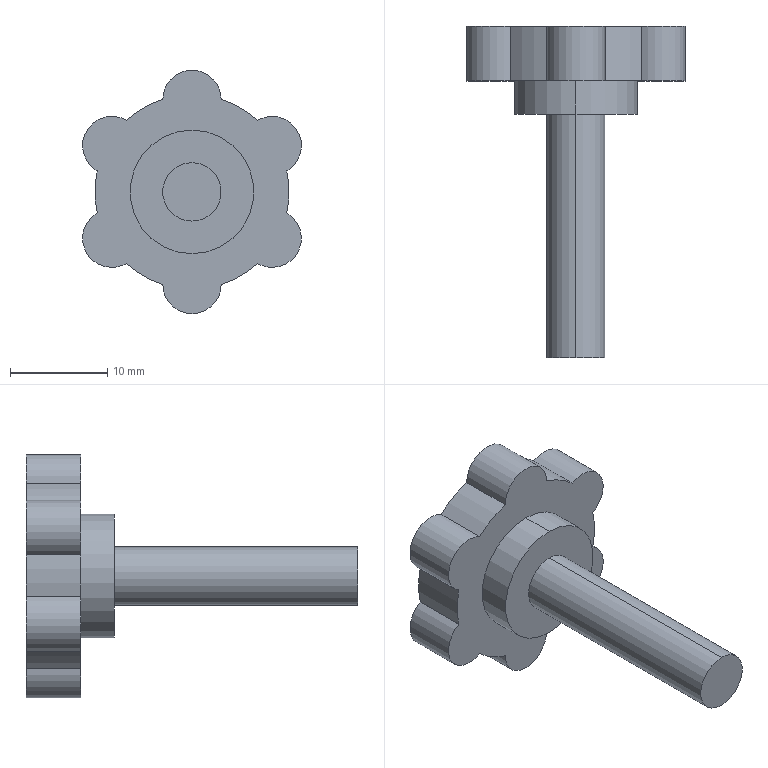Part | SolidWorks | features ICE 2, Extrusion 1 | 1 solid | 34 faces | box 22.455 x 34 x 25 mm | volume 3296 mm3 | cylinder 19 | plane 15 | commonest cylinder face diameters 6 x11 19.922 x6 12.7 x2
STEP:
#1=CARTESIAN_POINT('',(0.,-28.4,-3.));
#2=VERTEX_POINT('',#1);
#3=CARTESIAN_POINT('',(0.,-28.4,3.));
#4=VERTEX_POINT('',#3);
#5=CARTESIAN_POINT('',(0.,-28.4,0.));
#6=DIRECTION('',(0.,-1.,0.));
#7=DIRECTION('',(0.,0.,-1.));
#8=AXIS2_PLACEMENT_3D('',#5,#6,#7);
#9=CIRCLE('',#8,3.);
#10=EDGE_CURVE('',#2,#4,#9,.T.);
#11=ORIENTED_EDGE('',*,*,#10,.F.);
#12=CARTESIAN_POINT('',(0.,-3.4,-3.));
#13=VERTEX_POINT('',#12);
#14=CARTESIAN_POINT('',(0.,-28.4,-3.));
#15=DIRECTION('',(0.,1.,0.));
#16=VECTOR('',#15,1000.);
#17=LINE('',#14,#16);
#18=EDGE_CURVE('',#2,#13,#17,.T.);
#19=ORIENTED_EDGE('',*,*,#18,.T.);
#20=CARTESIAN_POINT('',(0.,-3.4,3.));
#21=VERTEX_POINT('',#20);
#22=CARTESIAN_POINT('',(0.,-3.4,0.));
#23=DIRECTION('',(0.,-1.,0.));
#24=DIRECTION('',(0.,0.,-1.));
#25=AXIS2_PLACEMENT_3D('',#22,#23,#24);
#26=CIRCLE('',#25,3.);
#27=EDGE_CURVE('',#13,#21,#26,.T.);
#28=ORIENTED_EDGE('',*,*,#27,.T.);
#29=CARTESIAN_POINT('',(0.,-28.4,3.));
#30=DIRECTION('',(0.,1.,0.));
#31=VECTOR('',#30,1000.);
#32=LINE('',#29,#31);
#33=EDGE_CURVE('',#4,#21,#32,.T.);
#34=ORIENTED_EDGE('',*,*,#33,.F.);
#35=EDGE_LOOP('',(#11,#19,#28,#34));
#36=FACE_OUTER_BOUND('',#35,.T.);
#37=CARTESIAN_POINT('',(0.,-28.4,0.));
#38=DIRECTION('',(0.,1.,0.));
#39=DIRECTION('',(0.,0.,1.));
#40=AXIS2_PLACEMENT_3D('',#37,#38,#39);
#41=CYLINDRICAL_SURFACE('',#40,3.);
#42=ADVANCED_FACE('',(#36),#41,.T.);
#43=CARTESIAN_POINT('',(0.,-3.4,-6.35));
#44=VERTEX_POINT('',#43);
#45=CARTESIAN_POINT('',(0.,-3.4,6.35));
#46=VERTEX_POINT('',#45);
#47=CARTESIAN_POINT('',(0.,-3.4,0.));
#48=DIRECTION('',(0.,-1.,0.));
#49=DIRECTION('',(0.,0.,-1.));
#50=AXIS2_PLACEMENT_3D('',#47,#48,#49);
#51=CIRCLE('',#50,6.35);
#52=EDGE_CURVE('',#44,#46,#51,.T.);
#53=ORIENTED_EDGE('',*,*,#52,.F.);
#54=CARTESIAN_POINT('',(0.,0.,-6.35));
#55=VERTEX_POINT('',#54);
#56=CARTESIAN_POINT('',(0.,-3.4,-6.35));
#57=DIRECTION('',(0.,1.,0.));
#58=VECTOR('',#57,1000.);
#59=LINE('',#56,#58);
#60=EDGE_CURVE('',#44,#55,#59,.T.);
#61=ORIENTED_EDGE('',*,*,#60,.T.);
#62=CARTESIAN_POINT('',(0.,0.,6.35));
#63=VERTEX_POINT('',#62);
#64=CARTESIAN_POINT('',(0.,0.,0.));
#65=DIRECTION('',(0.,-1.,0.));
#66=DIRECTION('',(0.,0.,1.));
#67=AXIS2_PLACEMENT_3D('',#64,#65,#66);
#68=CIRCLE('',#67,6.35);
#69=EDGE_CURVE('',#55,#63,#68,.T.);
#70=ORIENTED_EDGE('',*,*,#69,.T.);
#71=CARTESIAN_POINT('',(0.,-3.4,6.35));
#72=DIRECTION('',(0.,1.,0.));
#73=VECTOR('',#72,1000.);
#74=LINE('',#71,#73);
#75=EDGE_CURVE('',#46,#63,#74,.T.);
#76=ORIENTED_EDGE('',*,*,#75,.F.);
#77=EDGE_LOOP('',(#53,#61,#70,#76));
#78=FACE_OUTER_BOUND('',#77,.T.);
#79=CARTESIAN_POINT('',(0.,-3.4,0.));
#80=DIRECTION('',(0.,1.,0.));
#81=DIRECTION('',(0.,0.,1.));
#82=AXIS2_PLACEMENT_3D('',#79,#80,#81);
#83=CYLINDRICAL_SURFACE('',#82,6.35);
#84=ADVANCED_FACE('',(#78),#83,.T.);
#85=CARTESIAN_POINT('',(8.228,5.6,-7.751));
#86=VERTEX_POINT('',#85);
#87=CARTESIAN_POINT('',(6.728,5.6,-7.349));
#88=VERTEX_POINT('',#87);
#89=CARTESIAN_POINT('',(8.228,5.6,-4.751));
#90=DIRECTION('',(0.,1.,0.));
#91=DIRECTION('',(0.,0.,1.));
#92=AXIS2_PLACEMENT_3D('',#89,#90,#91);
#93=CIRCLE('',#92,3.);
#94=EDGE_CURVE('',#86,#88,#93,.T.);
#95=ORIENTED_EDGE('',*,*,#94,.F.);
#96=CARTESIAN_POINT('',(8.228,0.,-7.751));
#97=VERTEX_POINT('',#96);
#98=CARTESIAN_POINT('',(8.228,5.6,-7.751));
#99=DIRECTION('',(0.,-1.,0.));
#100=VECTOR('',#99,1000.);
#101=LINE('',#98,#100);
#102=EDGE_CURVE('',#86,#97,#101,.T.);
#103=ORIENTED_EDGE('',*,*,#102,.T.);
#104=CARTESIAN_POINT('',(6.728,0.,-7.349));
#105=VERTEX_POINT('',#104);
#106=CARTESIAN_POINT('',(8.228,0.,-4.751));
#107=DIRECTION('',(0.,1.,0.));
#108=DIRECTION('',(0.,0.,1.));
#109=AXIS2_PLACEMENT_3D('',#106,#107,#108);
#110=CIRCLE('',#109,3.);
#111=EDGE_CURVE('',#97,#105,#110,.T.);
#112=ORIENTED_EDGE('',*,*,#111,.T.);
#113=CARTESIAN_POINT('',(6.728,5.6,-7.349));
#114=DIRECTION('',(0.,-1.,0.));
#115=VECTOR('',#114,1000.);
#116=LINE('',#113,#115);
#117=EDGE_CURVE('',#88,#105,#116,.T.);
#118=ORIENTED_EDGE('',*,*,#117,.F.);
#119=EDGE_LOOP('',(#95,#103,#112,#118));
#120=FACE_OUTER_BOUND('',#119,.T.);
#121=CARTESIAN_POINT('',(8.228,5.6,-4.751));
#122=DIRECTION('',(0.,-1.,0.));
#123=DIRECTION('',(0.,0.,-1.));
#124=AXIS2_PLACEMENT_3D('',#121,#122,#123);
#125=CYLINDRICAL_SURFACE('',#124,3.);
#126=ADVANCED_FACE('',(#120),#125,.T.);
#127=CARTESIAN_POINT('',(-8.227,5.6,-7.749));
#128=VERTEX_POINT('',#127);
#129=CARTESIAN_POINT('',(-9.727,5.6,-2.151));
#130=VERTEX_POINT('',#129);
#131=CARTESIAN_POINT('',(-8.227,5.6,-4.749));
#132=DIRECTION('',(0.,1.,0.));
#133=DIRECTION('',(0.,0.,1.));
#134=AXIS2_PLACEMENT_3D('',#131,#132,#133);
#135=CIRCLE('',#134,3.);
#136=EDGE_CURVE('',#128,#130,#135,.T.);
#137=ORIENTED_EDGE('',*,*,#136,.F.);
#138=CARTESIAN_POINT('',(-8.227,0.,-7.749));
#139=VERTEX_POINT('',#138);
#140=CARTESIAN_POINT('',(-8.227,5.6,-7.749));
#141=DIRECTION('',(0.,-1.,0.));
#142=VECTOR('',#141,1000.);
#143=LINE('',#140,#142);
#144=EDGE_CURVE('',#128,#139,#143,.T.);
#145=ORIENTED_EDGE('',*,*,#144,.T.);
#146=CARTESIAN_POINT('',(-9.727,0.,-2.151));
#147=VERTEX_POINT('',#146);
#148=CARTESIAN_POINT('',(-8.227,0.,-4.749));
#149=DIRECTION('',(0.,1.,0.));
#150=DIRECTION('',(0.,0.,1.));
#151=AXIS2_PLACEMENT_3D('',#148,#149,#150);
#152=CIRCLE('',#151,3.);
#153=EDGE_CURVE('',#139,#147,#152,.T.);
#154=ORIENTED_EDGE('',*,*,#153,.T.);
#155=CARTESIAN_POINT('',(-9.727,5.6,-2.151));
#156=DIRECTION('',(0.,-1.,0.));
#157=VECTOR('',#156,1000.);
#158=LINE('',#155,#157);
#159=EDGE_CURVE('',#130,#147,#158,.T.);
#160=ORIENTED_EDGE('',*,*,#159,.F.);
#161=EDGE_LOOP('',(#137,#145,#154,#160));
#162=FACE_OUTER_BOUND('',#161,.T.);
#163=CARTESIAN_POINT('',(-8.227,5.6,-4.749));
#164=DIRECTION('',(0.,-1.,0.));
#165=DIRECTION('',(0.,0.,-1.));
#166=AXIS2_PLACEMENT_3D('',#163,#164,#165);
#167=CYLINDRICAL_SURFACE('',#166,3.);
#168=ADVANCED_FACE('',(#162),#167,.T.);
#169=CARTESIAN_POINT('',(0.,5.6,-12.5));
#170=VERTEX_POINT('',#169);
#171=CARTESIAN_POINT('',(-3.,5.6,-9.5));
#172=VERTEX_POINT('',#171);
#173=CARTESIAN_POINT('',(0.,5.6,-9.5));
#174=DIRECTION('',(0.,1.,0.));
#175=DIRECTION('',(0.,0.,1.));
#176=AXIS2_PLACEMENT_3D('',#173,#174,#175);
#177=CIRCLE('',#176,3.);
#178=EDGE_CURVE('',#170,#172,#177,.T.);
#179=ORIENTED_EDGE('',*,*,#178,.F.);
#180=CARTESIAN_POINT('',(0.,0.,-12.5));
#181=VERTEX_POINT('',#180);
#182=CARTESIAN_POINT('',(0.,5.6,-12.5));
#183=DIRECTION('',(0.,-1.,0.));
#184=VECTOR('',#183,1000.);
#185=LINE('',#182,#184);
#186=EDGE_CURVE('',#170,#181,#185,.T.);
#187=ORIENTED_EDGE('',*,*,#186,.T.);
#188=CARTESIAN_POINT('',(-3.,0.,-9.5));
#189=VERTEX_POINT('',#188);
#190=CARTESIAN_POINT('',(0.,0.,-9.5));
#191=DIRECTION('',(0.,1.,0.));
#192=DIRECTION('',(0.,0.,1.));
#193=AXIS2_PLACEMENT_3D('',#190,#191,#192);
#194=CIRCLE('',#193,3.);
#195=EDGE_CURVE('',#181,#189,#194,.T.);
#196=ORIENTED_EDGE('',*,*,#195,.T.);
#197=CARTESIAN_POINT('',(-3.,5.6,-9.5));
#198=DIRECTION('',(0.,-1.,0.));
#199=VECTOR('',#198,1000.);
#200=LINE('',#197,#199);
#201=EDGE_CURVE('',#172,#189,#200,.T.);
#202=ORIENTED_EDGE('',*,*,#201,.F.);
#203=EDGE_LOOP('',(#179,#187,#196,#202));
#204=FACE_OUTER_BOUND('',#203,.T.);
#205=CARTESIAN_POINT('',(0.,5.6,-9.5));
#206=DIRECTION('',(0.,-1.,0.));
#207=DIRECTION('',(0.,0.,-1.));
#208=AXIS2_PLACEMENT_3D('',#205,#206,#207);
#209=CYLINDRICAL_SURFACE('',#208,3.);
#210=ADVANCED_FACE('',(#204),#209,.T.);
#211=ORIENTED_EDGE('',*,*,#186,.F.);
#212=CARTESIAN_POINT('',(3.,5.6,-9.5));
#213=VERTEX_POINT('',#212);
#214=CARTESIAN_POINT('',(0.,5.6,-9.5));
#215=DIRECTION('',(0.,1.,0.));
#216=DIRECTION('',(0.,0.,1.));
#217=AXIS2_PLACEMENT_3D('',#214,#215,#216);
#218=CIRCLE('',#217,3.);
#219=EDGE_CURVE('',#213,#170,#218,.T.);
#220=ORIENTED_EDGE('',*,*,#219,.F.);
#221=CARTESIAN_POINT('',(3.,0.,-9.5));
#222=VERTEX_POINT('',#221);
#223=CARTESIAN_POINT('',(3.,5.6,-9.5));
#224=DIRECTION('',(0.,-1.,0.));
#225=VECTOR('',#224,1000.);
#226=LINE('',#223,#225);
#227=EDGE_CURVE('',#213,#222,#226,.T.);
#228=ORIENTED_EDGE('',*,*,#227,.T.);
#229=CARTESIAN_POINT('',(0.,0.,-9.5));
#230=DIRECTION('',(0.,1.,0.));
#231=DIRECTION('',(0.,0.,1.));
#232=AXIS2_PLACEMENT_3D('',#229,#230,#231);
#233=CIRCLE('',#232,3.);
#234=EDGE_CURVE('',#222,#181,#233,.T.);
#235=ORIENTED_EDGE('',*,*,#234,.T.);
#236=EDGE_LOOP('',(#211,#220,#228,#235));
#237=FACE_OUTER_BOUND('',#236,.T.);
#238=CARTESIAN_POINT('',(0.,5.6,-9.5));
#239=DIRECTION('',(0.,-1.,0.));
#240=DIRECTION('',(0.,0.,-1.));
#241=AXIS2_PLACEMENT_3D('',#238,#239,#240);
#242=CYLINDRICAL_SURFACE('',#241,3.);
#243=ADVANCED_FACE('',(#237),#242,.T.);
#244=CARTESIAN_POINT('',(-3.,0.,-9.499));
#245=VERTEX_POINT('',#244);
#246=CARTESIAN_POINT('',(-3.,0.,-9.499));
#247=DIRECTION('',(0.,0.,1.));
#248=VECTOR('',#247,1000.);
#249=LINE('',#246,#248);
#250=EDGE_CURVE('',#189,#245,#249,.T.);
#251=ORIENTED_EDGE('',*,*,#250,.T.);
#252=CARTESIAN_POINT('',(-3.,5.6,-9.499));
#253=VERTEX_POINT('',#252);
#254=CARTESIAN_POINT('',(-3.,5.6,-9.499));
#255=DIRECTION('',(0.,-1.,0.));
#256=VECTOR('',#255,1000.);
#257=LINE('',#254,#256);
#258=EDGE_CURVE('',#253,#245,#257,.T.);
#259=ORIENTED_EDGE('',*,*,#258,.F.);
#260=CARTESIAN_POINT('',(-3.,5.6,-9.499));
#261=DIRECTION('',(0.,0.,1.));
#262=VECTOR('',#261,1000.);
#263=LINE('',#260,#262);
#264=EDGE_CURVE('',#172,#253,#263,.T.);
#265=ORIENTED_EDGE('',*,*,#264,.F.);
#266=ORIENTED_EDGE('',*,*,#201,.T.);
#267=EDGE_LOOP('',(#251,#259,#265,#266));
#268=FACE_OUTER_BOUND('',#267,.T.);
#269=CARTESIAN_POINT('',(-3.,5.6,-9.499));
#270=DIRECTION('',(1.,0.,0.));
#271=DIRECTION('',(0.,0.,-1.));
#272=AXIS2_PLACEMENT_3D('',#269,#270,#271);
#273=PLANE('',#272);
#274=ADVANCED_FACE('',(#268),#273,.F.);
#275=CARTESIAN_POINT('',(-6.726,0.,-7.347));
#276=VERTEX_POINT('',#275);
#277=CARTESIAN_POINT('',(0.0015,0.,-0.000866));
#278=DIRECTION('',(0.,1.,0.));
#279=DIRECTION('',(0.,0.,1.));
#280=AXIS2_PLACEMENT_3D('',#277,#278,#279);
#281=CIRCLE('',#280,9.961);
#282=EDGE_CURVE('',#245,#276,#281,.T.);
#283=ORIENTED_EDGE('',*,*,#282,.T.);
#284=CARTESIAN_POINT('',(-6.726,5.6,-7.347));
#285=VERTEX_POINT('',#284);
#286=CARTESIAN_POINT('',(-6.726,5.6,-7.347));
#287=DIRECTION('',(0.,-1.,0.));
#288=VECTOR('',#287,1000.);
#289=LINE('',#286,#288);
#290=EDGE_CURVE('',#285,#276,#289,.T.);
#291=ORIENTED_EDGE('',*,*,#290,.F.);
#292=CARTESIAN_POINT('',(0.0015,5.6,-0.000866));
#293=DIRECTION('',(0.,1.,0.));
#294=DIRECTION('',(0.,0.,1.));
#295=AXIS2_PLACEMENT_3D('',#292,#293,#294);
#296=CIRCLE('',#295,9.961);
#297=EDGE_CURVE('',#253,#285,#296,.T.);
#298=ORIENTED_EDGE('',*,*,#297,.F.);
#299=ORIENTED_EDGE('',*,*,#258,.T.);
#300=EDGE_LOOP('',(#283,#291,#298,#299));
#301=FACE_OUTER_BOUND('',#300,.T.);
#302=CARTESIAN_POINT('',(0.0015,5.6,-0.000866));
#303=DIRECTION('',(0.,-1.,0.));
#304=DIRECTION('',(0.,0.,-1.));
#305=AXIS2_PLACEMENT_3D('',#302,#303,#304);
#306=CYLINDRICAL_SURFACE('',#305,9.961);
#307=ADVANCED_FACE('',(#301),#306,.T.);
#308=CARTESIAN_POINT('',(-6.727,0.,-7.347));
#309=VERTEX_POINT('',#308);
#310=CARTESIAN_POINT('',(-6.726,0.,-7.347));
#311=DIRECTION('',(-0.866,0.,-0.5));
#312=VECTOR('',#311,1000.);
#313=LINE('',#310,#312);
#314=EDGE_CURVE('',#276,#309,#313,.T.);
#315=ORIENTED_EDGE('',*,*,#314,.T.);
#316=CARTESIAN_POINT('',(-6.727,5.6,-7.347));
#317=VERTEX_POINT('',#316);
#318=CARTESIAN_POINT('',(-6.727,5.6,-7.347));
#319=DIRECTION('',(0.,-1.,0.));
#320=VECTOR('',#319,1000.);
#321=LINE('',#318,#320);
#322=EDGE_CURVE('',#317,#309,#321,.T.);
#323=ORIENTED_EDGE('',*,*,#322,.F.);
#324=CARTESIAN_POINT('',(-6.726,5.6,-7.347));
#325=DIRECTION('',(-0.866,0.,-0.5));
#326=VECTOR('',#325,1000.);
#327=LINE('',#324,#326);
#328=EDGE_CURVE('',#285,#317,#327,.T.);
#329=ORIENTED_EDGE('',*,*,#328,.F.);
#330=ORIENTED_EDGE('',*,*,#290,.T.);
#331=EDGE_LOOP('',(#315,#323,#329,#330));
#332=FACE_OUTER_BOUND('',#331,.T.);
#333=CARTESIAN_POINT('',(-6.726,5.6,-7.347));
#334=DIRECTION('',(-0.5,0.,0.866));
#335=DIRECTION('',(0.866,0.,0.5));
#336=AXIS2_PLACEMENT_3D('',#333,#334,#335);
#337=PLANE('',#336);
#338=ADVANCED_FACE('',(#332),#337,.F.);
#339=ORIENTED_EDGE('',*,*,#144,.F.);
#340=CARTESIAN_POINT('',(-8.227,5.6,-4.749));
#341=DIRECTION('',(0.,1.,0.));
#342=DIRECTION('',(0.,0.,1.));
#343=AXIS2_PLACEMENT_3D('',#340,#341,#342);
#344=CIRCLE('',#343,3.);
#345=EDGE_CURVE('',#317,#128,#344,.T.);
#346=ORIENTED_EDGE('',*,*,#345,.F.);
#347=ORIENTED_EDGE('',*,*,#322,.T.);
#348=CARTESIAN_POINT('',(-8.227,0.,-4.749));
#349=DIRECTION('',(0.,1.,0.));
#350=DIRECTION('',(0.,0.,1.));
#351=AXIS2_PLACEMENT_3D('',#348,#349,#350);
#352=CIRCLE('',#351,3.);
#353=EDGE_CURVE('',#309,#139,#352,.T.);
#354=ORIENTED_EDGE('',*,*,#353,.T.);
#355=EDGE_LOOP('',(#339,#346,#347,#354));
#356=FACE_OUTER_BOUND('',#355,.T.);
#357=CARTESIAN_POINT('',(-8.227,5.6,-4.749));
#358=DIRECTION('',(0.,-1.,0.));
#359=DIRECTION('',(0.,0.,-1.));
#360=AXIS2_PLACEMENT_3D('',#357,#358,#359);
#361=CYLINDRICAL_SURFACE('',#360,3.);
#362=ADVANCED_FACE('',(#356),#361,.T.);
#363=CARTESIAN_POINT('',(-9.725,0.,-2.15));
#364=VERTEX_POINT('',#363);
#365=CARTESIAN_POINT('',(-9.725,0.,-2.15));
#366=DIRECTION('',(0.866,0.,0.5));
#367=VECTOR('',#366,1000.);
#368=LINE('',#365,#367);
#369=EDGE_CURVE('',#147,#364,#368,.T.);
#370=ORIENTED_EDGE('',*,*,#369,.T.);
#371=CARTESIAN_POINT('',(-9.725,5.6,-2.15));
#372=VERTEX_POINT('',#371);
#373=CARTESIAN_POINT('',(-9.725,5.6,-2.15));
#374=DIRECTION('',(0.,-1.,0.));
#375=VECTOR('',#374,1000.);
#376=LINE('',#373,#375);
#377=EDGE_CURVE('',#372,#364,#376,.T.);
#378=ORIENTED_EDGE('',*,*,#377,.F.);
#379=CARTESIAN_POINT('',(-9.725,5.6,-2.15));
#380=DIRECTION('',(0.866,0.,0.5));
#381=VECTOR('',#380,1000.);
#382=LINE('',#379,#381);
#383=EDGE_CURVE('',#130,#372,#382,.T.);
#384=ORIENTED_EDGE('',*,*,#383,.F.);
#385=ORIENTED_EDGE('',*,*,#159,.T.);
#386=EDGE_LOOP('',(#370,#378,#384,#385));
#387=FACE_OUTER_BOUND('',#386,.T.);
#388=CARTESIAN_POINT('',(-9.725,5.6,-2.15));
#389=DIRECTION('',(0.5,0.,-0.866));
#390=DIRECTION('',(-0.866,0.,-0.5));
#391=AXIS2_PLACEMENT_3D('',#388,#389,#390);
#392=PLANE('',#391);
#393=ADVANCED_FACE('',(#387),#392,.F.);
#394=CARTESIAN_POINT('',(-9.724,0.,2.152));
#395=VERTEX_POINT('',#394);
#396=CARTESIAN_POINT('',(0.0015,0.,-0.000866));
#397=DIRECTION('',(0.,1.,0.));
#398=DIRECTION('',(0.,0.,1.));
#399=AXIS2_PLACEMENT_3D('',#396,#397,#398);
#400=CIRCLE('',#399,9.961);
#401=EDGE_CURVE('',#364,#395,#400,.T.);
#402=ORIENTED_EDGE('',*,*,#401,.T.);
#403=CARTESIAN_POINT('',(-9.724,5.6,2.152));
#404=VERTEX_POINT('',#403);
#405=CARTESIAN_POINT('',(-9.724,5.6,2.152));
#406=DIRECTION('',(0.,-1.,0.));
#407=VECTOR('',#406,1000.);
#408=LINE('',#405,#407);
#409=EDGE_CURVE('',#404,#395,#408,.T.);
#410=ORIENTED_EDGE('',*,*,#409,.F.);
#411=CARTESIAN_POINT('',(0.0015,5.6,-0.000866));
#412=DIRECTION('',(0.,1.,0.));
#413=DIRECTION('',(0.,0.,1.));
#414=AXIS2_PLACEMENT_3D('',#411,#412,#413);
#415=CIRCLE('',#414,9.961);
#416=EDGE_CURVE('',#372,#404,#415,.T.);
#417=ORIENTED_EDGE('',*,*,#416,.F.);
#418=ORIENTED_EDGE('',*,*,#377,.T.);
#419=EDGE_LOOP('',(#402,#410,#417,#418));
#420=FACE_OUTER_BOUND('',#419,.T.);
#421=CARTESIAN_POINT('',(0.0015,5.6,-0.000866));
#422=DIRECTION('',(0.,-1.,0.));
#423=DIRECTION('',(0.,0.,-1.));
#424=AXIS2_PLACEMENT_3D('',#421,#422,#423);
#425=CYLINDRICAL_SURFACE('',#424,9.961);
#426=ADVANCED_FACE('',(#420),#425,.T.);
#427=CARTESIAN_POINT('',(-9.726,0.,2.153));
#428=VERTEX_POINT('',#427);
#429=CARTESIAN_POINT('',(-9.724,0.,2.152));
#430=DIRECTION('',(-0.866,0.,0.5));
#431=VECTOR('',#430,1000.);
#432=LINE('',#429,#431);
#433=EDGE_CURVE('',#395,#428,#432,.T.);
#434=ORIENTED_EDGE('',*,*,#433,.T.);
#435=CARTESIAN_POINT('',(-9.726,5.6,2.153));
#436=VERTEX_POINT('',#435);
#437=CARTESIAN_POINT('',(-9.726,5.6,2.153));
#438=DIRECTION('',(0.,-1.,0.));
#439=VECTOR('',#438,1000.);
#440=LINE('',#437,#439);
#441=EDGE_CURVE('',#436,#428,#440,.T.);
#442=ORIENTED_EDGE('',*,*,#441,.F.);
#443=CARTESIAN_POINT('',(-9.724,5.6,2.152));
#444=DIRECTION('',(-0.866,0.,0.5));
#445=VECTOR('',#444,1000.);
#446=LINE('',#443,#445);
#447=EDGE_CURVE('',#404,#436,#446,.T.);
#448=ORIENTED_EDGE('',*,*,#447,.F.);
#449=ORIENTED_EDGE('',*,*,#409,.T.);
#450=EDGE_LOOP('',(#434,#442,#448,#449));
#451=FACE_OUTER_BOUND('',#450,.T.);
#452=CARTESIAN_POINT('',(-9.724,5.6,2.152));
#453=DIRECTION('',(0.5,0.,0.866));
#454=DIRECTION('',(0.866,0.,-0.5));
#455=AXIS2_PLACEMENT_3D('',#452,#453,#454);
#456=PLANE('',#455);
#457=ADVANCED_FACE('',(#451),#456,.F.);
#458=CARTESIAN_POINT('',(-6.726,0.,7.349));
#459=VERTEX_POINT('',#458);
#460=CARTESIAN_POINT('',(-8.226,0.,4.751));
#461=DIRECTION('',(0.,1.,0.));
#462=DIRECTION('',(0.,0.,1.));
#463=AXIS2_PLACEMENT_3D('',#460,#461,#462);
#464=CIRCLE('',#463,3.);
#465=EDGE_CURVE('',#428,#459,#464,.T.);
#466=ORIENTED_EDGE('',*,*,#465,.T.);
#467=CARTESIAN_POINT('',(-6.726,5.6,7.349));
#468=VERTEX_POINT('',#467);
#469=CARTESIAN_POINT('',(-6.726,5.6,7.349));
#470=DIRECTION('',(0.,-1.,0.));
#471=VECTOR('',#470,1000.);
#472=LINE('',#469,#471);
#473=EDGE_CURVE('',#468,#459,#472,.T.);
#474=ORIENTED_EDGE('',*,*,#473,.F.);
#475=CARTESIAN_POINT('',(-8.226,5.6,4.751));
#476=DIRECTION('',(0.,1.,0.));
#477=DIRECTION('',(0.,0.,1.));
#478=AXIS2_PLACEMENT_3D('',#475,#476,#477);
#479=CIRCLE('',#478,3.);
#480=EDGE_CURVE('',#436,#468,#479,.T.);
#481=ORIENTED_EDGE('',*,*,#480,.F.);
#482=ORIENTED_EDGE('',*,*,#441,.T.);
#483=EDGE_LOOP('',(#466,#474,#481,#482));
#484=FACE_OUTER_BOUND('',#483,.T.);
#485=CARTESIAN_POINT('',(-8.226,5.6,4.751));
#486=DIRECTION('',(0.,-1.,0.));
#487=DIRECTION('',(0.,0.,-1.));
#488=AXIS2_PLACEMENT_3D('',#485,#486,#487);
#489=CYLINDRICAL_SURFACE('',#488,3.);
#490=ADVANCED_FACE('',(#484),#489,.T.);
#491=CARTESIAN_POINT('',(-6.723,0.,7.348));
#492=VERTEX_POINT('',#491);
#493=CARTESIAN_POINT('',(-6.723,0.,7.348));
#494=DIRECTION('',(0.866,0.,-0.5));
#495=VECTOR('',#494,1000.);
#496=LINE('',#493,#495);
#497=EDGE_CURVE('',#459,#492,#496,.T.);
#498=ORIENTED_EDGE('',*,*,#497,.T.);
#499=CARTESIAN_POINT('',(-6.723,5.6,7.348));
#500=VERTEX_POINT('',#499);
#501=CARTESIAN_POINT('',(-6.723,5.6,7.348));
#502=DIRECTION('',(0.,-1.,0.));
#503=VECTOR('',#502,1000.);
#504=LINE('',#501,#503);
#505=EDGE_CURVE('',#500,#492,#504,.T.);
#506=ORIENTED_EDGE('',*,*,#505,.F.);
#507=CARTESIAN_POINT('',(-6.723,5.6,7.348));
#508=DIRECTION('',(0.866,0.,-0.5));
#509=VECTOR('',#508,1000.);
#510=LINE('',#507,#509);
#511=EDGE_CURVE('',#468,#500,#510,.T.);
#512=ORIENTED_EDGE('',*,*,#511,.F.);
#513=ORIENTED_EDGE('',*,*,#473,.T.);
#514=EDGE_LOOP('',(#498,#506,#512,#513));
#515=FACE_OUTER_BOUND('',#514,.T.);
#516=CARTESIAN_POINT('',(-6.723,5.6,7.348));
#517=DIRECTION('',(-0.5,0.,-0.866));
#518=DIRECTION('',(-0.866,0.,0.5));
#519=AXIS2_PLACEMENT_3D('',#516,#517,#518);
#520=PLANE('',#519);
#521=ADVANCED_FACE('',(#515),#520,.F.);
#522=CARTESIAN_POINT('',(-2.998,0.,9.498));
#523=VERTEX_POINT('',#522);
#524=CARTESIAN_POINT('',(0.0015,0.,-0.000866));
#525=DIRECTION('',(0.,1.,0.));
#526=DIRECTION('',(0.,0.,1.));
#527=AXIS2_PLACEMENT_3D('',#524,#525,#526);
#528=CIRCLE('',#527,9.961);
#529=EDGE_CURVE('',#492,#523,#528,.T.);
#530=ORIENTED_EDGE('',*,*,#529,.T.);
#531=CARTESIAN_POINT('',(-2.998,5.6,9.498));
#532=VERTEX_POINT('',#531);
#533=CARTESIAN_POINT('',(-2.998,5.6,9.498));
#534=DIRECTION('',(0.,-1.,0.));
#535=VECTOR('',#534,1000.);
#536=LINE('',#533,#535);
#537=EDGE_CURVE('',#532,#523,#536,.T.);
#538=ORIENTED_EDGE('',*,*,#537,.F.);
#539=CARTESIAN_POINT('',(0.0015,5.6,-0.000866));
#540=DIRECTION('',(0.,1.,0.));
#541=DIRECTION('',(0.,0.,1.));
#542=AXIS2_PLACEMENT_3D('',#539,#540,#541);
#543=CIRCLE('',#542,9.961);
#544=EDGE_CURVE('',#500,#532,#543,.T.);
#545=ORIENTED_EDGE('',*,*,#544,.F.);
#546=ORIENTED_EDGE('',*,*,#505,.T.);
#547=EDGE_LOOP('',(#530,#538,#545,#546));
#548=FACE_OUTER_BOUND('',#547,.T.);
#549=CARTESIAN_POINT('',(0.0015,5.6,-0.000866));
#550=DIRECTION('',(0.,-1.,0.));
#551=DIRECTION('',(0.,0.,-1.));
#552=AXIS2_PLACEMENT_3D('',#549,#550,#551);
#553=CYLINDRICAL_SURFACE('',#552,9.961);
#554=ADVANCED_FACE('',(#548),#553,.T.);
#555=CARTESIAN_POINT('',(-2.998,0.,9.5));
#556=VERTEX_POINT('',#555);
#557=CARTESIAN_POINT('',(-2.998,0.,9.498));
#558=DIRECTION('',(0.,0.,1.));
#559=VECTOR('',#558,1000.);
#560=LINE('',#557,#559);
#561=EDGE_CURVE('',#523,#556,#560,.T.);
#562=ORIENTED_EDGE('',*,*,#561,.T.);
#563=CARTESIAN_POINT('',(-2.998,5.6,9.5));
#564=VERTEX_POINT('',#563);
#565=CARTESIAN_POINT('',(-2.998,5.6,9.5));
#566=DIRECTION('',(0.,-1.,0.));
#567=VECTOR('',#566,1000.);
#568=LINE('',#565,#567);
#569=EDGE_CURVE('',#564,#556,#568,.T.);
#570=ORIENTED_EDGE('',*,*,#569,.F.);
#571=CARTESIAN_POINT('',(-2.998,5.6,9.498));
#572=DIRECTION('',(0.,0.,1.));
#573=VECTOR('',#572,1000.);
#574=LINE('',#571,#573);
#575=EDGE_CURVE('',#532,#564,#574,.T.);
#576=ORIENTED_EDGE('',*,*,#575,.F.);
#577=ORIENTED_EDGE('',*,*,#537,.T.);
#578=EDGE_LOOP('',(#562,#570,#576,#577));
#579=FACE_OUTER_BOUND('',#578,.T.);
#580=CARTESIAN_POINT('',(-2.998,5.6,9.498));
#581=DIRECTION('',(1.,0.,0.));
#582=DIRECTION('',(0.,0.,-1.));
#583=AXIS2_PLACEMENT_3D('',#580,#581,#582);
#584=PLANE('',#583);
#585=ADVANCED_FACE('',(#579),#584,.F.);
#586=CARTESIAN_POINT('',(3.002,0.,9.5));
#587=VERTEX_POINT('',#586);
#588=CARTESIAN_POINT('',(0.002,0.,9.5));
#589=DIRECTION('',(0.,1.,0.));
#590=DIRECTION('',(0.,0.,1.));
#591=AXIS2_PLACEMENT_3D('',#588,#589,#590);
#592=CIRCLE('',#591,3.);
#593=EDGE_CURVE('',#556,#587,#592,.T.);
#594=ORIENTED_EDGE('',*,*,#593,.T.);
#595=CARTESIAN_POINT('',(3.002,5.6,9.5));
#596=VERTEX_POINT('',#595);
#597=CARTESIAN_POINT('',(3.002,5.6,9.5));
#598=DIRECTION('',(0.,-1.,0.));
#599=VECTOR('',#598,1000.);
#600=LINE('',#597,#599);
#601=EDGE_CURVE('',#596,#587,#600,.T.);
#602=ORIENTED_EDGE('',*,*,#601,.F.);
#603=CARTESIAN_POINT('',(0.002,5.6,9.5));
#604=DIRECTION('',(0.,1.,0.));
#605=DIRECTION('',(0.,0.,1.));
#606=AXIS2_PLACEMENT_3D('',#603,#604,#605);
#607=CIRCLE('',#606,3.);
#608=EDGE_CURVE('',#564,#596,#607,.T.);
#609=ORIENTED_EDGE('',*,*,#608,.F.);
#610=ORIENTED_EDGE('',*,*,#569,.T.);
#611=EDGE_LOOP('',(#594,#602,#609,#610));
#612=FACE_OUTER_BOUND('',#611,.T.);
#613=CARTESIAN_POINT('',(0.002,5.6,9.5));
#614=DIRECTION('',(0.,-1.,0.));
#615=DIRECTION('',(0.,0.,-1.));
#616=AXIS2_PLACEMENT_3D('',#613,#614,#615);
#617=CYLINDRICAL_SURFACE('',#616,3.);
#618=ADVANCED_FACE('',(#612),#617,.T.);
#619=CARTESIAN_POINT('',(3.002,0.,9.498));
#620=VERTEX_POINT('',#619);
#621=CARTESIAN_POINT('',(3.002,0.,9.498));
#622=DIRECTION('',(0.,0.,-1.));
#623=VECTOR('',#622,1000.);
#624=LINE('',#621,#623);
#625=EDGE_CURVE('',#587,#620,#624,.T.);
#626=ORIENTED_EDGE('',*,*,#625,.T.);
#627=CARTESIAN_POINT('',(3.002,5.6,9.498));
#628=VERTEX_POINT('',#627);
#629=CARTESIAN_POINT('',(3.002,5.6,9.498));
#630=DIRECTION('',(0.,-1.,0.));
#631=VECTOR('',#630,1000.);
#632=LINE('',#629,#631);
#633=EDGE_CURVE('',#628,#620,#632,.T.);
#634=ORIENTED_EDGE('',*,*,#633,.F.);
#635=CARTESIAN_POINT('',(3.002,5.6,9.498));
#636=DIRECTION('',(0.,0.,-1.));
#637=VECTOR('',#636,1000.);
#638=LINE('',#635,#637);
#639=EDGE_CURVE('',#596,#628,#638,.T.);
#640=ORIENTED_EDGE('',*,*,#639,.F.);
#641=ORIENTED_EDGE('',*,*,#601,.T.);
#642=EDGE_LOOP('',(#626,#634,#640,#641));
#643=FACE_OUTER_BOUND('',#642,.T.);
#644=CARTESIAN_POINT('',(3.002,5.6,9.498));
#645=DIRECTION('',(-1.,0.,0.));
#646=DIRECTION('',(0.,0.,1.));
#647=AXIS2_PLACEMENT_3D('',#644,#645,#646);
#648=PLANE('',#647);
#649=ADVANCED_FACE('',(#643),#648,.F.);
#650=CARTESIAN_POINT('',(6.728,0.,7.347));
#651=VERTEX_POINT('',#650);
#652=CARTESIAN_POINT('',(0.0015,0.,-0.000866));
#653=DIRECTION('',(0.,1.,0.));
#654=DIRECTION('',(0.,0.,1.));
#655=AXIS2_PLACEMENT_3D('',#652,#653,#654);
#656=CIRCLE('',#655,9.961);
#657=EDGE_CURVE('',#620,#651,#656,.T.);
#658=ORIENTED_EDGE('',*,*,#657,.T.);
#659=CARTESIAN_POINT('',(6.728,5.6,7.347));
#660=VERTEX_POINT('',#659);
#661=CARTESIAN_POINT('',(6.728,5.6,7.347));
#662=DIRECTION('',(0.,-1.,0.));
#663=VECTOR('',#662,1000.);
#664=LINE('',#661,#663);
#665=EDGE_CURVE('',#660,#651,#664,.T.);
#666=ORIENTED_EDGE('',*,*,#665,.F.);
#667=CARTESIAN_POINT('',(0.0015,5.6,-0.000866));
#668=DIRECTION('',(0.,1.,0.));
#669=DIRECTION('',(0.,0.,1.));
#670=AXIS2_PLACEMENT_3D('',#667,#668,#669);
#671=CIRCLE('',#670,9.961);
#672=EDGE_CURVE('',#628,#660,#671,.T.);
#673=ORIENTED_EDGE('',*,*,#672,.F.);
#674=ORIENTED_EDGE('',*,*,#633,.T.);
#675=EDGE_LOOP('',(#658,#666,#673,#674));
#676=FACE_OUTER_BOUND('',#675,.T.);
#677=CARTESIAN_POINT('',(0.0015,5.6,-0.000866));
#678=DIRECTION('',(0.,-1.,0.));
#679=DIRECTION('',(0.,0.,-1.));
#680=AXIS2_PLACEMENT_3D('',#677,#678,#679);
#681=CYLINDRICAL_SURFACE('',#680,9.961);
#682=ADVANCED_FACE('',(#676),#681,.T.);
#683=CARTESIAN_POINT('',(6.729,0.,7.347));
#684=VERTEX_POINT('',#683);
#685=CARTESIAN_POINT('',(6.728,0.,7.347));
#686=DIRECTION('',(0.866,0.,0.5));
#687=VECTOR('',#686,1000.);
#688=LINE('',#685,#687);
#689=EDGE_CURVE('',#651,#684,#688,.T.);
#690=ORIENTED_EDGE('',*,*,#689,.T.);
#691=CARTESIAN_POINT('',(6.729,5.6,7.347));
#692=VERTEX_POINT('',#691);
#693=CARTESIAN_POINT('',(6.729,5.6,7.347));
#694=DIRECTION('',(0.,-1.,0.));
#695=VECTOR('',#694,1000.);
#696=LINE('',#693,#695);
#697=EDGE_CURVE('',#692,#684,#696,.T.);
#698=ORIENTED_EDGE('',*,*,#697,.F.);
#699=CARTESIAN_POINT('',(6.728,5.6,7.347));
#700=DIRECTION('',(0.866,0.,0.5));
#701=VECTOR('',#700,1000.);
#702=LINE('',#699,#701);
#703=EDGE_CURVE('',#660,#692,#702,.T.);
#704=ORIENTED_EDGE('',*,*,#703,.F.);
#705=ORIENTED_EDGE('',*,*,#665,.T.);
#706=EDGE_LOOP('',(#690,#698,#704,#705));
#707=FACE_OUTER_BOUND('',#706,.T.);
#708=CARTESIAN_POINT('',(6.728,5.6,7.347));
#709=DIRECTION('',(0.5,0.,-0.866));
#710=DIRECTION('',(-0.866,0.,-0.5));
#711=AXIS2_PLACEMENT_3D('',#708,#709,#710);
#712=PLANE('',#711);
#713=ADVANCED_FACE('',(#707),#712,.F.);
#714=CARTESIAN_POINT('',(9.729,0.,2.151));
#715=VERTEX_POINT('',#714);
#716=CARTESIAN_POINT('',(8.229,0.,4.749));
#717=DIRECTION('',(0.,1.,0.));
#718=DIRECTION('',(0.,0.,1.));
#719=AXIS2_PLACEMENT_3D('',#716,#717,#718);
#720=CIRCLE('',#719,3.);
#721=EDGE_CURVE('',#684,#715,#720,.T.);
#722=ORIENTED_EDGE('',*,*,#721,.T.);
#723=CARTESIAN_POINT('',(9.729,5.6,2.151));
#724=VERTEX_POINT('',#723);
#725=CARTESIAN_POINT('',(9.729,5.6,2.151));
#726=DIRECTION('',(0.,-1.,0.));
#727=VECTOR('',#726,1000.);
#728=LINE('',#725,#727);
#729=EDGE_CURVE('',#724,#715,#728,.T.);
#730=ORIENTED_EDGE('',*,*,#729,.F.);
#731=CARTESIAN_POINT('',(8.229,5.6,4.749));
#732=DIRECTION('',(0.,1.,0.));
#733=DIRECTION('',(0.,0.,1.));
#734=AXIS2_PLACEMENT_3D('',#731,#732,#733);
#735=CIRCLE('',#734,3.);
#736=EDGE_CURVE('',#692,#724,#735,.T.);
#737=ORIENTED_EDGE('',*,*,#736,.F.);
#738=ORIENTED_EDGE('',*,*,#697,.T.);
#739=EDGE_LOOP('',(#722,#730,#737,#738));
#740=FACE_OUTER_BOUND('',#739,.T.);
#741=CARTESIAN_POINT('',(8.229,5.6,4.749));
#742=DIRECTION('',(0.,-1.,0.));
#743=DIRECTION('',(0.,0.,-1.));
#744=AXIS2_PLACEMENT_3D('',#741,#742,#743);
#745=CYLINDRICAL_SURFACE('',#744,3.);
#746=ADVANCED_FACE('',(#740),#745,.T.);
#747=CARTESIAN_POINT('',(9.728,0.,2.15));
#748=VERTEX_POINT('',#747);
#749=CARTESIAN_POINT('',(9.728,0.,2.15));
#750=DIRECTION('',(-0.866,0.,-0.5));
#751=VECTOR('',#750,1000.);
#752=LINE('',#749,#751);
#753=EDGE_CURVE('',#715,#748,#752,.T.);
#754=ORIENTED_EDGE('',*,*,#753,.T.);
#755=CARTESIAN_POINT('',(9.728,5.6,2.15));
#756=VERTEX_POINT('',#755);
#757=CARTESIAN_POINT('',(9.728,5.6,2.15));
#758=DIRECTION('',(0.,-1.,0.));
#759=VECTOR('',#758,1000.);
#760=LINE('',#757,#759);
#761=EDGE_CURVE('',#756,#748,#760,.T.);
#762=ORIENTED_EDGE('',*,*,#761,.F.);
#763=CARTESIAN_POINT('',(9.728,5.6,2.15));
#764=DIRECTION('',(-0.866,0.,-0.5));
#765=VECTOR('',#764,1000.);
#766=LINE('',#763,#765);
#767=EDGE_CURVE('',#724,#756,#766,.T.);
#768=ORIENTED_EDGE('',*,*,#767,.F.);
#769=ORIENTED_EDGE('',*,*,#729,.T.);
#770=EDGE_LOOP('',(#754,#762,#768,#769));
#771=FACE_OUTER_BOUND('',#770,.T.);
#772=CARTESIAN_POINT('',(9.728,5.6,2.15));
#773=DIRECTION('',(-0.5,0.,0.866));
#774=DIRECTION('',(0.866,0.,0.5));
#775=AXIS2_PLACEMENT_3D('',#772,#773,#774);
#776=PLANE('',#775);
#777=ADVANCED_FACE('',(#771),#776,.F.);
#778=CARTESIAN_POINT('',(9.727,0.,-2.153));
#779=VERTEX_POINT('',#778);
#780=CARTESIAN_POINT('',(0.0015,0.,-0.000866));
#781=DIRECTION('',(0.,1.,0.));
#782=DIRECTION('',(0.,0.,1.));
#783=AXIS2_PLACEMENT_3D('',#780,#781,#782);
#784=CIRCLE('',#783,9.961);
#785=EDGE_CURVE('',#748,#779,#784,.T.);
#786=ORIENTED_EDGE('',*,*,#785,.T.);
#787=CARTESIAN_POINT('',(9.727,5.6,-2.153));
#788=VERTEX_POINT('',#787);
#789=CARTESIAN_POINT('',(9.727,5.6,-2.153));
#790=DIRECTION('',(0.,-1.,0.));
#791=VECTOR('',#790,1000.);
#792=LINE('',#789,#791);
#793=EDGE_CURVE('',#788,#779,#792,.T.);
#794=ORIENTED_EDGE('',*,*,#793,.F.);
#795=CARTESIAN_POINT('',(0.0015,5.6,-0.000866));
#796=DIRECTION('',(0.,1.,0.));
#797=DIRECTION('',(0.,0.,1.));
#798=AXIS2_PLACEMENT_3D('',#795,#796,#797);
#799=CIRCLE('',#798,9.961);
#800=EDGE_CURVE('',#756,#788,#799,.T.);
#801=ORIENTED_EDGE('',*,*,#800,.F.);
#802=ORIENTED_EDGE('',*,*,#761,.T.);
#803=EDGE_LOOP('',(#786,#794,#801,#802));
#804=FACE_OUTER_BOUND('',#803,.T.);
#805=CARTESIAN_POINT('',(0.0015,5.6,-0.000866));
#806=DIRECTION('',(0.,-1.,0.));
#807=DIRECTION('',(0.,0.,-1.));
#808=AXIS2_PLACEMENT_3D('',#805,#806,#807);
#809=CYLINDRICAL_SURFACE('',#808,9.961);
#810=ADVANCED_FACE('',(#804),#809,.T.);
#811=CARTESIAN_POINT('',(9.728,0.,-2.153));
#812=VERTEX_POINT('',#811);
#813=CARTESIAN_POINT('',(9.727,0.,-2.153));
#814=DIRECTION('',(0.866,0.,-0.5));
#815=VECTOR('',#814,1000.);
#816=LINE('',#813,#815);
#817=EDGE_CURVE('',#779,#812,#816,.T.);
#818=ORIENTED_EDGE('',*,*,#817,.T.);
#819=CARTESIAN_POINT('',(9.728,5.6,-2.153));
#820=VERTEX_POINT('',#819);
#821=CARTESIAN_POINT('',(9.728,5.6,-2.153));
#822=DIRECTION('',(0.,-1.,0.));
#823=VECTOR('',#822,1000.);
#824=LINE('',#821,#823);
#825=EDGE_CURVE('',#820,#812,#824,.T.);
#826=ORIENTED_EDGE('',*,*,#825,.F.);
#827=CARTESIAN_POINT('',(9.727,5.6,-2.153));
#828=DIRECTION('',(0.866,0.,-0.5));
#829=VECTOR('',#828,1000.);
#830=LINE('',#827,#829);
#831=EDGE_CURVE('',#788,#820,#830,.T.);
#832=ORIENTED_EDGE('',*,*,#831,.F.);
#833=ORIENTED_EDGE('',*,*,#793,.T.);
#834=EDGE_LOOP('',(#818,#826,#832,#833));
#835=FACE_OUTER_BOUND('',#834,.T.);
#836=CARTESIAN_POINT('',(9.727,5.6,-2.153));
#837=DIRECTION('',(-0.5,0.,-0.866));
#838=DIRECTION('',(-0.866,0.,0.5));
#839=AXIS2_PLACEMENT_3D('',#836,#837,#838);
#840=PLANE('',#839);
#841=ADVANCED_FACE('',(#835),#840,.F.);
#842=ORIENTED_EDGE('',*,*,#102,.F.);
#843=CARTESIAN_POINT('',(8.228,5.6,-4.751));
#844=DIRECTION('',(0.,1.,0.));
#845=DIRECTION('',(0.,0.,1.));
#846=AXIS2_PLACEMENT_3D('',#843,#844,#845);
#847=CIRCLE('',#846,3.);
#848=EDGE_CURVE('',#820,#86,#847,.T.);
#849=ORIENTED_EDGE('',*,*,#848,.F.);
#850=ORIENTED_EDGE('',*,*,#825,.T.);
#851=CARTESIAN_POINT('',(8.228,0.,-4.751));
#852=DIRECTION('',(0.,1.,0.));
#853=DIRECTION('',(0.,0.,1.));
#854=AXIS2_PLACEMENT_3D('',#851,#852,#853);
#855=CIRCLE('',#854,3.);
#856=EDGE_CURVE('',#812,#97,#855,.T.);
#857=ORIENTED_EDGE('',*,*,#856,.T.);
#858=EDGE_LOOP('',(#842,#849,#850,#857));
#859=FACE_OUTER_BOUND('',#858,.T.);
#860=CARTESIAN_POINT('',(8.228,5.6,-4.751));
#861=DIRECTION('',(0.,-1.,0.));
#862=DIRECTION('',(0.,0.,-1.));
#863=AXIS2_PLACEMENT_3D('',#860,#861,#862);
#864=CYLINDRICAL_SURFACE('',#863,3.);
#865=ADVANCED_FACE('',(#859),#864,.T.);
#866=CARTESIAN_POINT('',(6.727,0.,-7.349));
#867=VERTEX_POINT('',#866);
#868=CARTESIAN_POINT('',(6.727,0.,-7.349));
#869=DIRECTION('',(-0.866,0.,0.5));
#870=VECTOR('',#869,1000.);
#871=LINE('',#868,#870);
#872=EDGE_CURVE('',#105,#867,#871,.T.);
#873=ORIENTED_EDGE('',*,*,#872,.T.);
#874=CARTESIAN_POINT('',(6.727,5.6,-7.349));
#875=VERTEX_POINT('',#874);
#876=CARTESIAN_POINT('',(6.727,5.6,-7.349));
#877=DIRECTION('',(0.,-1.,0.));
#878=VECTOR('',#877,1000.);
#879=LINE('',#876,#878);
#880=EDGE_CURVE('',#875,#867,#879,.T.);
#881=ORIENTED_EDGE('',*,*,#880,.F.);
#882=CARTESIAN_POINT('',(6.727,5.6,-7.349));
#883=DIRECTION('',(-0.866,0.,0.5));
#884=VECTOR('',#883,1000.);
#885=LINE('',#882,#884);
#886=EDGE_CURVE('',#88,#875,#885,.T.);
#887=ORIENTED_EDGE('',*,*,#886,.F.);
#888=ORIENTED_EDGE('',*,*,#117,.T.);
#889=EDGE_LOOP('',(#873,#881,#887,#888));
#890=FACE_OUTER_BOUND('',#889,.T.);
#891=CARTESIAN_POINT('',(6.727,5.6,-7.349));
#892=DIRECTION('',(0.5,0.,0.866));
#893=DIRECTION('',(0.866,0.,-0.5));
#894=AXIS2_PLACEMENT_3D('',#891,#892,#893);
#895=PLANE('',#894);
#896=ADVANCED_FACE('',(#890),#895,.F.);
#897=CARTESIAN_POINT('',(0.0015,0.,-0.000866));
#898=DIRECTION('',(0.,1.,0.));
#899=DIRECTION('',(0.,0.,1.));
#900=AXIS2_PLACEMENT_3D('',#897,#898,#899);
#901=CIRCLE('',#900,9.961);
#902=EDGE_CURVE('',#867,#222,#901,.T.);
#903=ORIENTED_EDGE('',*,*,#902,.T.);
#904=ORIENTED_EDGE('',*,*,#227,.F.);
#905=CARTESIAN_POINT('',(0.0015,5.6,-0.000866));
#906=DIRECTION('',(0.,1.,0.));
#907=DIRECTION('',(0.,0.,1.));
#908=AXIS2_PLACEMENT_3D('',#905,#906,#907);
#909=CIRCLE('',#908,9.961);
#910=EDGE_CURVE('',#875,#213,#909,.T.);
#911=ORIENTED_EDGE('',*,*,#910,.F.);
#912=ORIENTED_EDGE('',*,*,#880,.T.);
#913=EDGE_LOOP('',(#903,#904,#911,#912));
#914=FACE_OUTER_BOUND('',#913,.T.);
#915=CARTESIAN_POINT('',(0.0015,5.6,-0.000866));
#916=DIRECTION('',(0.,-1.,0.));
#917=DIRECTION('',(0.,0.,-1.));
#918=AXIS2_PLACEMENT_3D('',#915,#916,#917);
#919=CYLINDRICAL_SURFACE('',#918,9.961);
#920=ADVANCED_FACE('',(#914),#919,.T.);
#921=ORIENTED_EDGE('',*,*,#219,.T.);
#922=ORIENTED_EDGE('',*,*,#178,.T.);
#923=ORIENTED_EDGE('',*,*,#264,.T.);
#924=ORIENTED_EDGE('',*,*,#297,.T.);
#925=ORIENTED_EDGE('',*,*,#328,.T.);
#926=ORIENTED_EDGE('',*,*,#345,.T.);
#927=ORIENTED_EDGE('',*,*,#136,.T.);
#928=ORIENTED_EDGE('',*,*,#383,.T.);
#929=ORIENTED_EDGE('',*,*,#416,.T.);
#930=ORIENTED_EDGE('',*,*,#447,.T.);
#931=ORIENTED_EDGE('',*,*,#480,.T.);
#932=ORIENTED_EDGE('',*,*,#511,.T.);
#933=ORIENTED_EDGE('',*,*,#544,.T.);
#934=ORIENTED_EDGE('',*,*,#575,.T.);
#935=ORIENTED_EDGE('',*,*,#608,.T.);
#936=ORIENTED_EDGE('',*,*,#639,.T.);
#937=ORIENTED_EDGE('',*,*,#672,.T.);
#938=ORIENTED_EDGE('',*,*,#703,.T.);
#939=ORIENTED_EDGE('',*,*,#736,.T.);
#940=ORIENTED_EDGE('',*,*,#767,.T.);
#941=ORIENTED_EDGE('',*,*,#800,.T.);
#942=ORIENTED_EDGE('',*,*,#831,.T.);
#943=ORIENTED_EDGE('',*,*,#848,.T.);
#944=ORIENTED_EDGE('',*,*,#94,.T.);
#945=ORIENTED_EDGE('',*,*,#886,.T.);
#946=ORIENTED_EDGE('',*,*,#910,.T.);
#947=EDGE_LOOP('',(#921,#922,#923,#924,#925,#926,#927,#928,#929,#930,#931,#932,#933,#934,#935,#936,#937,#938,#939,#940,#941,#942,#943,#944,#945,#946));
#948=FACE_OUTER_BOUND('',#947,.T.);
#949=CARTESIAN_POINT('',(0.,5.6,-9.5));
#950=DIRECTION('',(0.,1.,0.));
#951=DIRECTION('',(0.,0.,1.));
#952=AXIS2_PLACEMENT_3D('',#949,#950,#951);
#953=PLANE('',#952);
#954=ADVANCED_FACE('',(#948),#953,.T.);
#955=CARTESIAN_POINT('',(0.,0.,0.));
#956=DIRECTION('',(0.,-1.,0.));
#957=DIRECTION('',(0.,0.,1.));
#958=AXIS2_PLACEMENT_3D('',#955,#956,#957);
#959=CIRCLE('',#958,6.35);
#960=EDGE_CURVE('',#63,#55,#959,.T.);
#961=ORIENTED_EDGE('',*,*,#960,.F.);
#962=ORIENTED_EDGE('',*,*,#69,.F.);
#963=EDGE_LOOP('',(#961,#962));
#964=FACE_BOUND('',#963,.T.);
#965=ORIENTED_EDGE('',*,*,#234,.F.);
#966=ORIENTED_EDGE('',*,*,#902,.F.);
#967=ORIENTED_EDGE('',*,*,#872,.F.);
#968=ORIENTED_EDGE('',*,*,#111,.F.);
#969=ORIENTED_EDGE('',*,*,#856,.F.);
#970=ORIENTED_EDGE('',*,*,#817,.F.);
#971=ORIENTED_EDGE('',*,*,#785,.F.);
#972=ORIENTED_EDGE('',*,*,#753,.F.);
#973=ORIENTED_EDGE('',*,*,#721,.F.);
#974=ORIENTED_EDGE('',*,*,#689,.F.);
#975=ORIENTED_EDGE('',*,*,#657,.F.);
#976=ORIENTED_EDGE('',*,*,#625,.F.);
#977=ORIENTED_EDGE('',*,*,#593,.F.);
#978=ORIENTED_EDGE('',*,*,#561,.F.);
#979=ORIENTED_EDGE('',*,*,#529,.F.);
#980=ORIENTED_EDGE('',*,*,#497,.F.);
#981=ORIENTED_EDGE('',*,*,#465,.F.);
#982=ORIENTED_EDGE('',*,*,#433,.F.);
#983=ORIENTED_EDGE('',*,*,#401,.F.);
#984=ORIENTED_EDGE('',*,*,#369,.F.);
#985=ORIENTED_EDGE('',*,*,#153,.F.);
#986=ORIENTED_EDGE('',*,*,#353,.F.);
#987=ORIENTED_EDGE('',*,*,#314,.F.);
#988=ORIENTED_EDGE('',*,*,#282,.F.);
#989=ORIENTED_EDGE('',*,*,#250,.F.);
#990=ORIENTED_EDGE('',*,*,#195,.F.);
#991=EDGE_LOOP('',(#965,#966,#967,#968,#969,#970,#971,#972,#973,#974,#975,#976,#977,#978,#979,#980,#981,#982,#983,#984,#985,#986,#987,#988,#989,#990));
#992=FACE_OUTER_BOUND('',#991,.T.);
#993=CARTESIAN_POINT('',(0.,0.,-9.5));
#994=DIRECTION('',(0.,1.,0.));
#995=DIRECTION('',(0.,0.,1.));
#996=AXIS2_PLACEMENT_3D('',#993,#994,#995);
#997=PLANE('',#996);
#998=ADVANCED_FACE('',(#964,#992),#997,.F.);
#999=ORIENTED_EDGE('',*,*,#60,.F.);
#1000=CARTESIAN_POINT('',(0.,-3.4,0.));
#1001=DIRECTION('',(0.,-1.,0.));
#1002=DIRECTION('',(0.,0.,-1.));
#1003=AXIS2_PLACEMENT_3D('',#1000,#1001,#1002);
#1004=CIRCLE('',#1003,6.35);
#1005=EDGE_CURVE('',#46,#44,#1004,.T.);
#1006=ORIENTED_EDGE('',*,*,#1005,.F.);
#1007=ORIENTED_EDGE('',*,*,#75,.T.);
#1008=ORIENTED_EDGE('',*,*,#960,.T.);
#1009=EDGE_LOOP('',(#999,#1006,#1007,#1008));
#1010=FACE_OUTER_BOUND('',#1009,.T.);
#1011=CARTESIAN_POINT('',(0.,-3.4,0.));
#1012=DIRECTION('',(0.,1.,0.));
#1013=DIRECTION('',(0.,0.,1.));
#1014=AXIS2_PLACEMENT_3D('',#1011,#1012,#1013);
#1015=CYLINDRICAL_SURFACE('',#1014,6.35);
#1016=ADVANCED_FACE('',(#1010),#1015,.T.);
#1017=CARTESIAN_POINT('',(0.,-3.4,0.));
#1018=DIRECTION('',(0.,-1.,0.));
#1019=DIRECTION('',(0.,0.,-1.));
#1020=AXIS2_PLACEMENT_3D('',#1017,#1018,#1019);
#1021=CIRCLE('',#1020,3.);
#1022=EDGE_CURVE('',#21,#13,#1021,.T.);
#1023=ORIENTED_EDGE('',*,*,#1022,.F.);
#1024=ORIENTED_EDGE('',*,*,#27,.F.);
#1025=EDGE_LOOP('',(#1023,#1024));
#1026=FACE_BOUND('',#1025,.T.);
#1027=ORIENTED_EDGE('',*,*,#1005,.T.);
#1028=ORIENTED_EDGE('',*,*,#52,.T.);
#1029=EDGE_LOOP('',(#1027,#1028));
#1030=FACE_OUTER_BOUND('',#1029,.T.);
#1031=CARTESIAN_POINT('',(0.,-3.4,0.));
#1032=DIRECTION('',(0.,-1.,0.));
#1033=DIRECTION('',(0.,0.,-1.));
#1034=AXIS2_PLACEMENT_3D('',#1031,#1032,#1033);
#1035=PLANE('',#1034);
#1036=ADVANCED_FACE('',(#1026,#1030),#1035,.T.);
#1037=ORIENTED_EDGE('',*,*,#18,.F.);
#1038=CARTESIAN_POINT('',(0.,-28.4,0.));
#1039=DIRECTION('',(0.,-1.,0.));
#1040=DIRECTION('',(0.,0.,-1.));
#1041=AXIS2_PLACEMENT_3D('',#1038,#1039,#1040);
#1042=CIRCLE('',#1041,3.);
#1043=EDGE_CURVE('',#4,#2,#1042,.T.);
#1044=ORIENTED_EDGE('',*,*,#1043,.F.);
#1045=ORIENTED_EDGE('',*,*,#33,.T.);
#1046=ORIENTED_EDGE('',*,*,#1022,.T.);
#1047=EDGE_LOOP('',(#1037,#1044,#1045,#1046));
#1048=FACE_OUTER_BOUND('',#1047,.T.);
#1049=CARTESIAN_POINT('',(0.,-28.4,0.));
#1050=DIRECTION('',(0.,1.,0.));
#1051=DIRECTION('',(0.,0.,1.));
#1052=AXIS2_PLACEMENT_3D('',#1049,#1050,#1051);
#1053=CYLINDRICAL_SURFACE('',#1052,3.);
#1054=ADVANCED_FACE('',(#1048),#1053,.T.);
#1055=ORIENTED_EDGE('',*,*,#1043,.T.);
#1056=ORIENTED_EDGE('',*,*,#10,.T.);
#1057=EDGE_LOOP('',(#1055,#1056));
#1058=FACE_OUTER_BOUND('',#1057,.T.);
#1059=CARTESIAN_POINT('',(0.,-28.4,0.));
#1060=DIRECTION('',(0.,-1.,0.));
#1061=DIRECTION('',(0.,0.,-1.));
#1062=AXIS2_PLACEMENT_3D('',#1059,#1060,#1061);
#1063=PLANE('',#1062);
#1064=ADVANCED_FACE('',(#1058),#1063,.T.);
#1065=CLOSED_SHELL('',(#42,#84,#126,#168,#210,#243,#274,#307,#338,#362,#393,#426,#457,#490,#521,#554,#585,#618,#649,#682,#713,#746,#777,#810,#841,#865,#896,#920,#954,#998,#1016,#1036,#1054,#1064));
#1066=MANIFOLD_SOLID_BREP('',#1065);
#1067=CARTESIAN_POINT('',(0.,0.,0.));
#1068=DIRECTION('',(0.,0.,1.));
#1069=DIRECTION('',(1.,0.,0.));
#1070=AXIS2_PLACEMENT_3D('',#1067,#1068,#1069);
#1071=(LENGTH_UNIT()NAMED_UNIT(*)SI_UNIT(.MILLI.,.METRE.));
#1072=UNCERTAINTY_MEASURE_WITH_UNIT(LENGTH_MEASURE(0.00001),#1071,'','');
#1073=(NAMED_UNIT(*)PLANE_ANGLE_UNIT()SI_UNIT($,.RADIAN.));
#1074=(NAMED_UNIT(*)SI_UNIT($,.STERADIAN.)SOLID_ANGLE_UNIT());
#1075=(GEOMETRIC_REPRESENTATION_CONTEXT(3)GLOBAL_UNCERTAINTY_ASSIGNED_CONTEXT((#1072))GLOBAL_UNIT_ASSIGNED_CONTEXT((#1071,#1073,#1074))REPRESENTATION_CONTEXT('',''));
#1076=ADVANCED_BREP_SHAPE_REPRESENTATION('',(#1066,#1070),#1075);